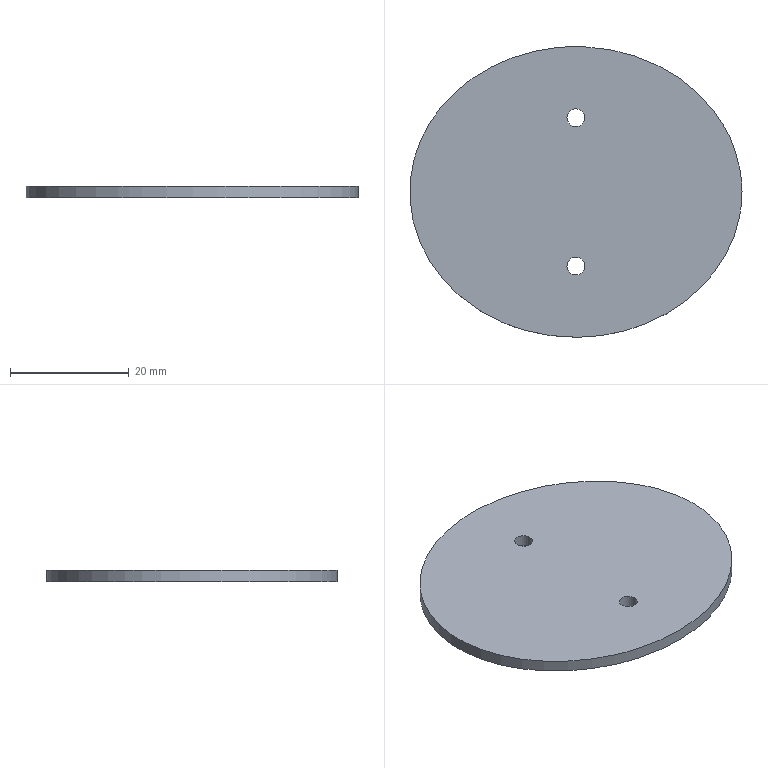Part | NX | features DATUM_CSYS 2, EXTRUDE 1, SKETCH 1 | 1 solid | 5 faces | box 56 x 49 x 2 mm | volume 4282 mm3 | cylinder 2 | plane 2 | spline 1 | commonest cylinder face diameters 3 x2